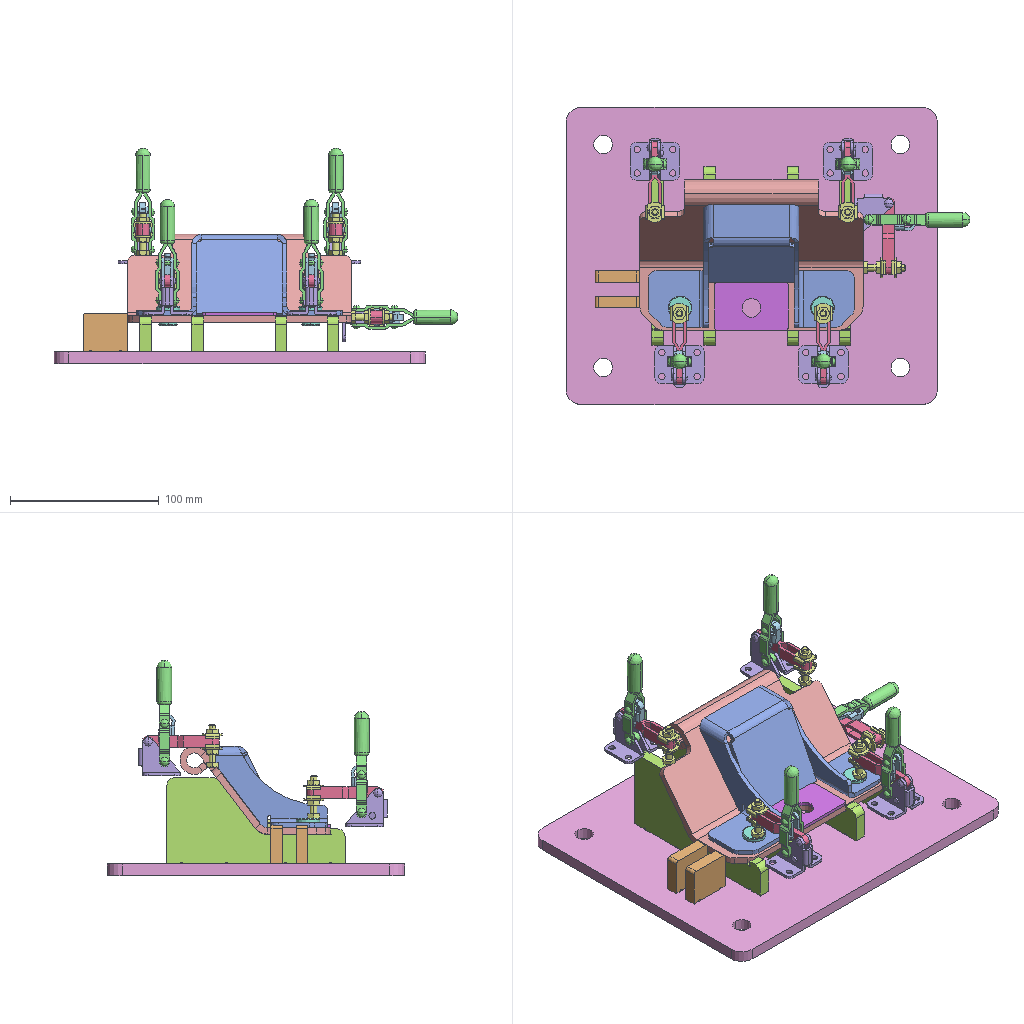Assembly | SolidWorks | 8 different items | 17 placed | box 272 x 200 x 145 mm
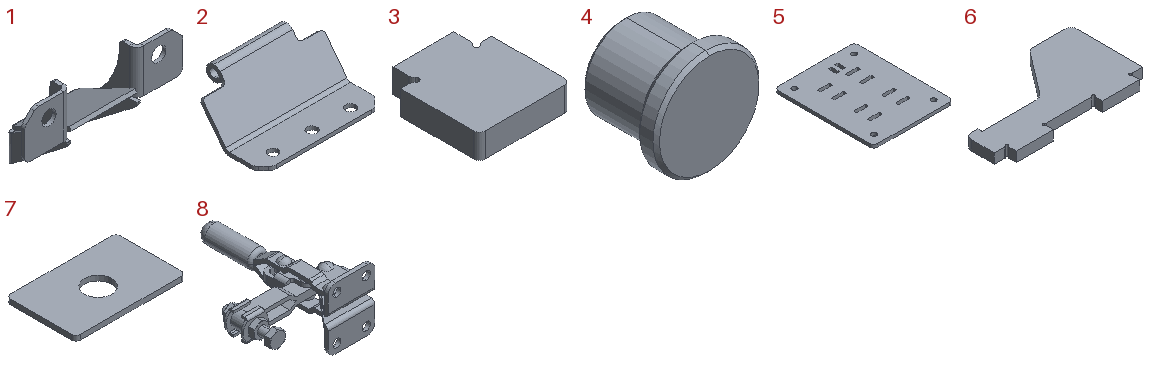Parts list (item | quantity | size | volume | features):
1 | x1 | 138.4 x 54.6 x 82.5 mm | 33246 mm3 | features Fillet 3, ICE 3, EdgeFlange 2, Chamfer 1, FlatPattern 1, SMBaseFlange 1, SheetMetal 1
2 | x1 | 150.4 x 101.2 x 59.2 mm | 84882 mm3 | features Fillet 2, ICE 2, Chamfer 1, FlatPattern 1, SMBaseFlange 1, SheetMetal 1
3 | x2 | 30 x 33.5 x 8 mm | 7383 mm3 | features FlatPattern 1, SMBaseFlange 1, SheetMetal 1
4 | x2 | 16 x 13 x 16 mm | 1794 mm3 | features Chamfer 1, Revolution 1
5 | x1 | 200 x 250 x 8 mm | 377466 mm3 | features FlatPattern 1, SMBaseFlange 1, SheetMetal 1
6 | x4 | 120 x 65.5 x 8 mm | 37548 mm3 | features FlatPattern 1, SMBaseFlange 1, SheetMetal 1
7 | x1 | 50 x 31.95 x 2.3 mm | 3384 mm3 | features FlatPattern 1, SMBaseFlange 1, SheetMetal 1
8 | x5 | 56.45 x 77.62 x 33.3 mm | 10418 mm3 | features BaseBody 5
Mates (type | each side: item.copy, entity, surface, feature):
Coincident | 2.1 face plane Base-Flange1 | 1.1 face plane Edge-Flange2
Concentric | 2.1 face cylinder Cut-Extrude3 | 1.1 face cylinder Cut-Extrude3 | 2 times
InPlace | 1.1 face plane Base-Flange1 | 6.1 plane
InPlace | 6.2 face plane Base-Flange1 | 5.1 plane
InPlace | 4.1 plane | assembly plane
InPlace | 3.1 plane | assembly plane
Coincident | 4.1 face plane Revolve1 | 8.1 face plane PN_0001 vertical flange-seat quick clamp [PN_0002].step-1/_PN_0002(bolt).step-1-solid1
Coincident | 2.1 edge | 8.2 face plane PN_0001 vertical flange-seat quick clamp [PN_0002].step-1/_PN_0002(bolt).step-1-solid1
Coincident | 2.1 face plane Base-Flange1 | 8.3 face plane PN_0001 vertical flange-seat quick clamp [PN_0002].step-1/_PN_0002(bolt).step-1-solid1
InPlace | 2.1 face plane Base-Flange1 | 7.1 plane